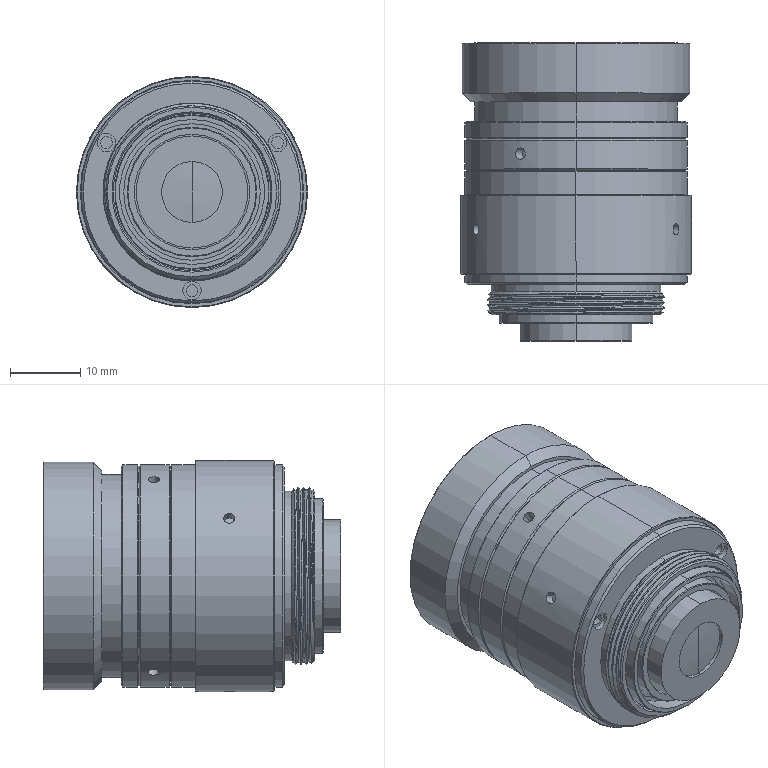Part | SolidWorks | features BaseBody 16 | 13 solids | 345 faces | box 33 x 42.54 x 33 mm | volume 18425 mm3 | cylinder 178 | plane 74 | cone 70 | spline 15 | sphere 8 | commonest cylinder face diameters 1.6 x12 27.5 x10 27 x8 31.8 x8 1.7 x6 2.6 x6